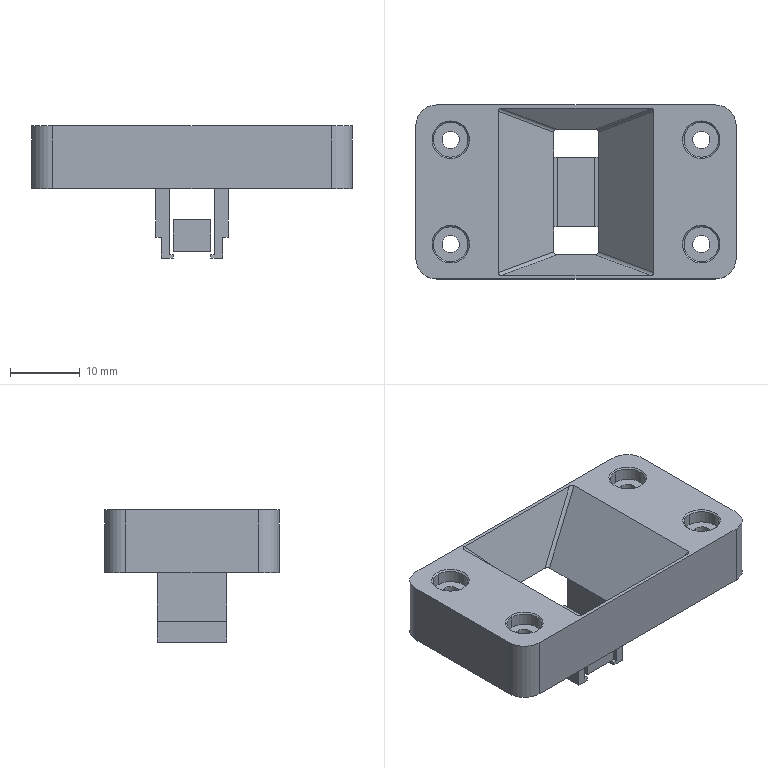Part | 2 solids | 70 faces | box 46 x 25 x 19 mm | volume 7793 mm3 | plane 38 | cylinder 24 | cone 8 | commonest cylinder face diameters 2.5 x8 5 x8 1 x4 6 x4